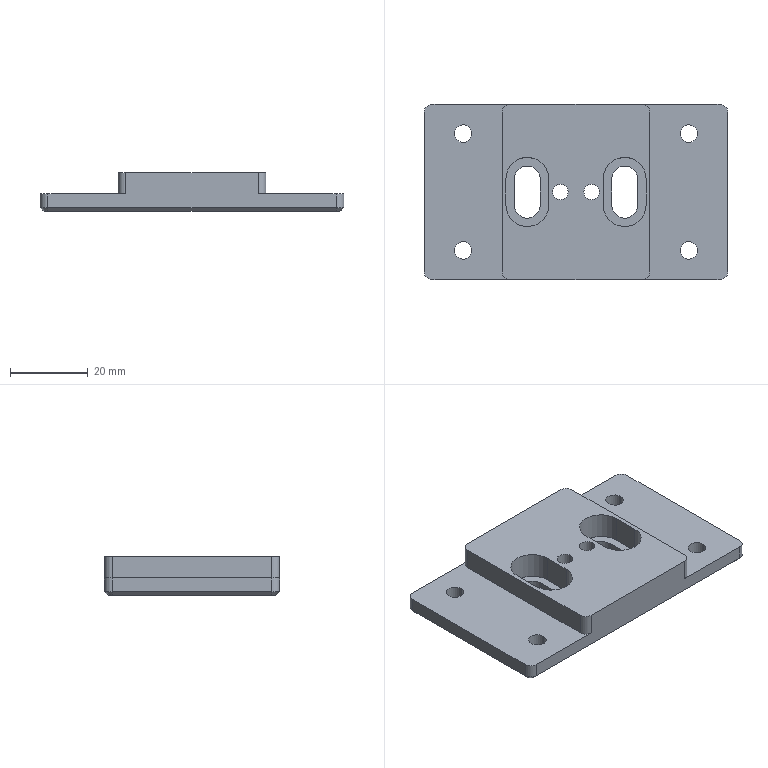NC program | NX | posted with a generic post | part box 78 x 45 x 10 mm
Whole program:
N10 G17 G21 G94 G90
(FLOOR_WALL_COPY , TOOL : D63)
N12 T01 M6
N14 G54
N16 G17 G0 G90 X-73.5 Y0. S6500 M3
N18 G43 Z30. H1
N20 Z4.
N22 G94 G1 Z1. F1250.
N24 X-70.5
N26 X70.5
N28 X73.5
N30 Z4.
N32 G0 Z30.
N34 X-73.5
N36 Z3.
N38 G1 Z0.
N40 X-70.5
N42 X70.5
N44 X73.5
N46 Z3.
N48 G0 Z30.
N50 M5
(ZLEVEL_PROFILE_1_COPY_1_COPY_COPY_1 , TOOL : D6A45)
N52 T07 M6
N54 G54
N56 G17 G0 G90 X-29.042 Y-15.081 S9500 M3
N58 G43 Z30. H7
N60 Z0.
N62 G94 G1 Z-1. F1000.
N64 X-29.52 Y-15.991
N66 G3 X-29. Y-16.291 R0.6
N68 X-27.709 Y-15. R1.291
N70 X-29. Y-16.291 R-1.291
N72 X-28.48 Y-15.991 R0.6
N74 G1 X-28.958 Y-15.081
N76 Z0.
N78 G0 Z30.
N80 X4. Y1.041
N82 Z1.
N84 G1 Z-1.
N86 G3 X2.959 Y0. R1.041
N88 X4. Y1.041 R-1.041
N90 X3.48 Y0.741 R0.6
N92 G1 Z0.
N94 G0 Z30.
N96 X-4. Y1.041
N98 Z1.
N100 G1 Z-1.
N102 G3 X-5.041 Y0. R1.041
N104 X-4. Y1.041 R-1.041
N106 X-4.52 Y0.741 R0.6
N108 G1 Z0.
N110 G0 Z30.
N112 X29.042 Y15.081
N114 Z0.
N116 G1 Z-1.
N118 X29.52 Y15.991
N120 G3 X29. Y16.291 R0.6
N122 X27.709 Y15. R1.291
N124 X29. Y16.291 R-1.291
N126 X28.48 Y15.991 R0.6
N128 G1 X28.958 Y15.081
N130 Z0.
N132 G0 Z30.
N134 X-28.958
N136 Z0.
N138 G1 Z-1.
N140 X-28.48 Y15.991
N142 G3 X-29. Y16.291 R0.6
N144 X-30.291 Y15. R1.291
N146 X-29. Y16.291 R-1.291
N148 X-29.52 Y15.991 R0.6
N150 G1 X-29.042 Y15.081
N152 Z0.
N154 G0 Z30.
N156 X11.394 Y3.682
N158 Z0.
N160 G1 Z-1.
N162 X10.459 Y3.92
N164 G3 X10.159 Y3.4 R0.6
N166 G1 Y-3.4
N168 G3 X12.5 Y-5.741 R2.341
N170 X14.841 Y-3.4 R2.341
N172 G1 Y3.4
N174 G3 X12.5 Y5.741 R2.341
N176 X10.159 Y3.4 R2.341
N178 X10.459 Y2.88 R0.6
N180 G1 X11.359 Y2.361
N182 Z0.
N184 G0 Z30.
N186 X-11.394 Y-3.682
N188 Z0.
N190 G1 Z-1.
N192 X-10.459 Y-3.92
N194 G3 X-10.159 Y-3.4 R0.6
N196 G1 Y3.4
N198 G3 X-12.5 Y5.741 R2.341
N200 X-14.841 Y3.4 R2.341
N202 G1 Y-3.4
N204 G3 X-12.5 Y-5.741 R2.341
N206 X-10.159 Y-3.4 R2.341
N208 X-10.459 Y-2.88 R0.6
N210 G1 X-11.359 Y-2.361
N212 Z0.
N214 G0 Z30.
N216 X28.958 Y-15.081
N218 Z0.
N220 G1 Z-1.
N222 X28.48 Y-15.991
N224 G3 X29. Y-16.291 R0.6
N226 X30.291 Y-15. R1.291
N228 X29. Y-16.291 R-1.291
N230 X29.52 Y-15.991 R0.6
N232 G1 X29.042 Y-15.081
N234 Z0.
N236 G0 Z30.
(ZLEVEL_PROFILE_1_COPY_1_COPY_COPY_1_COPY , TOOL : D6A45)
N238 X37.973 Y-24.586
N240 Z-1.
N242 G1 Z-2.
N244 X37.52 Y-23.8
N246 G3 X37. Y-23.5 R0.6
N248 G1 X-37.
N250 G2 X-40. Y-20.5 R3.
N252 G1 Y20.5
N254 G2 X-37. Y23.5 R3.
N256 G1 X37.
N258 G2 X40. Y20.5 R3.
N260 G1 Y-20.5
N262 G2 X37. Y-23.5 R3.
N264 G3 X36.48 Y-23.8 R0.6
N266 G1 X35.961 Y-24.7
N268 Z-1.
N270 G0 Z30.
N272 M5
N274 M2